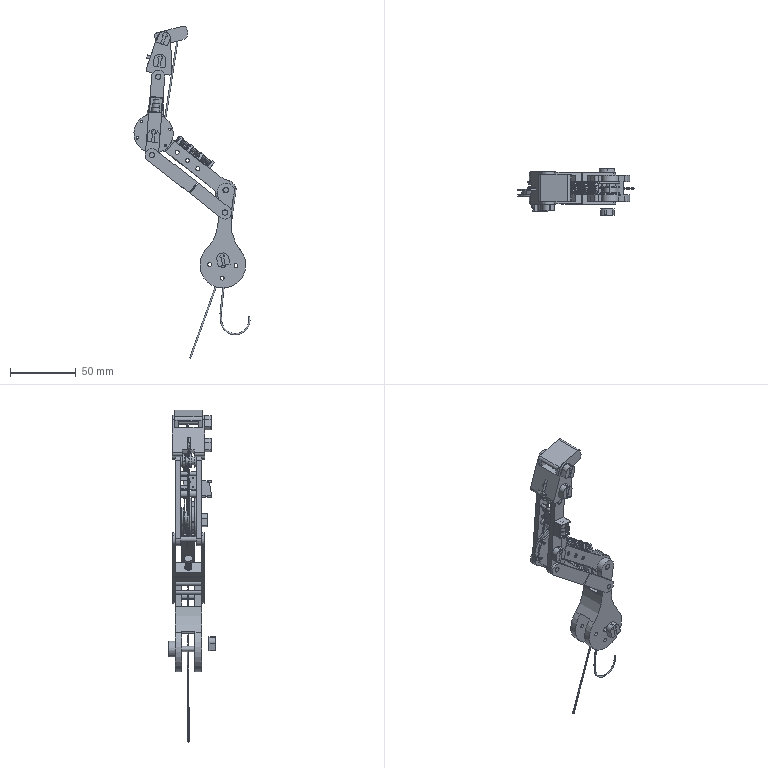Part | SolidWorks | features ReferencePattern 4, CompositeCurve 2, Cut 1, MirrorCompFeat 1 | 35 solids | 832 faces | box 88.567 x 35.49 x 253.176 mm | volume 52231 mm3 | cylinder 537 | plane 259 | torus 24 | spline 8 | cone 4 | commonest cylinder face diameters 3.2 x108 4 x82 6.748 x51 3 x48 9 x48 10 x47